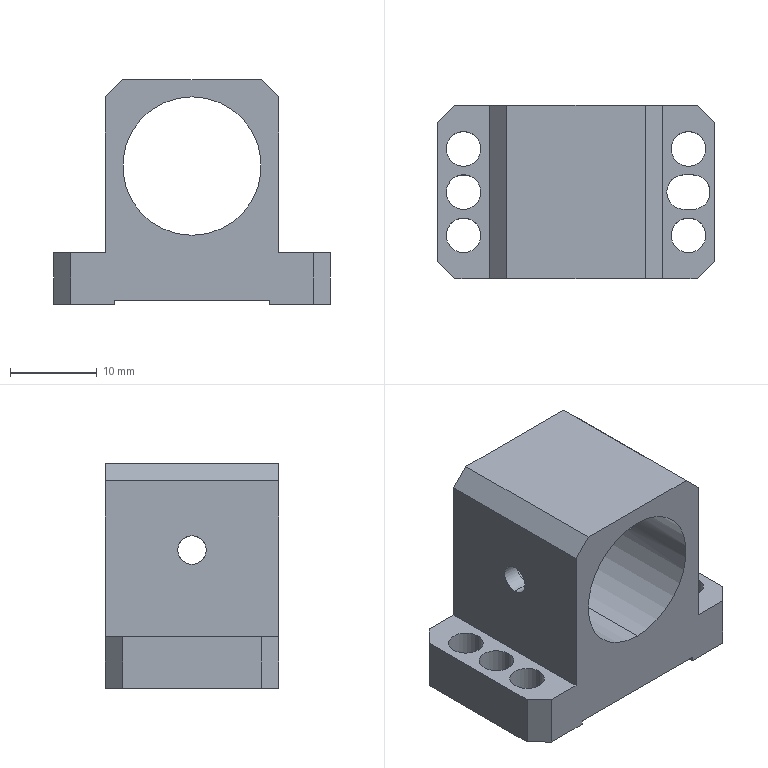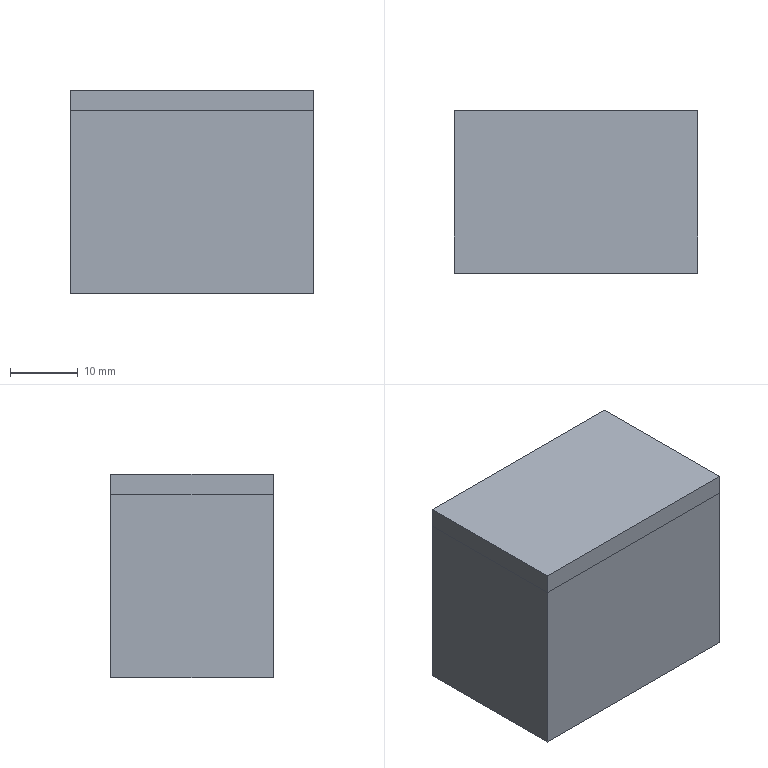CAM job | NX | 3+2 milling, drilling | part box 32 x 20 x 26 mm | stock box 36 x 24 x 30 mm
Tools:
number,name,description,diameter,corner_radius,flute_length,length,flutes
11,D10JING,Milling Tool-5 Parameters,10.0,0.0,50.0,75.0,2
10,D10,Milling Tool-5 Parameters,10.0,0.0,50.0,75.0,2
5,D4R0.5,Milling Tool-5 Parameters,4.0,0.5,50.0,75.0,2
7,D6A45,Milling Tool-5 Parameters,6.0,0.0,50.0,75.0,2
14,4.0ZT,Drilling Tool,4.0,0.0,35.0,50.0,2
3,D3,Milling Tool-5 Parameters,3.0,0.0,50.0,75.0,2
Operations:
program,operation,operation_type,tool,method,geometry_group,spindle_rpm,surface_speed,feed_per_tooth,feed_cut,feed_plunge,cut_length_mm,path_length_mm,cut_time_min,machine_time_min
1,FLOOR_WALL,VolumeBased25DMillingOperation,D10JING,METHOD,A,9500.0,298.0,0.0658,1250.0,100.0,315.997,369.997,0.2528,0.2582
1,ZLEVEL_PROFILE,ZLevelMilling,D10,METHOD,A,9500.0,298.0,0.1579,3000.0,1000.0,6899.193,6982.193,2.325,2.333
1,FLOOR_WALL_1,VolumeBased25DMillingOperation,D10,METHOD,A,9500.0,179.0,0.1316,2500.0,1000.0,4110.117,4436.557,2.005,2.037
1,ZLEVEL_PROFILE_COPY_1,ZLevelMilling,D10JING,METHOD,A,9500.0,298.0,0.0632,1200.0,1000.0,278.136,473.496,0.2331,0.2527
1,FLOOR_WALL_1_1,VolumeBased25DMillingOperation,D10JING,METHOD,A,9500.0,298.0,0.0658,1250.0,100.0,254.567,587.327,0.2037,0.2369
1,ZLEVEL_PROFILE_1,ZLevelMilling,D4R0.5,METHOD,A,9500.0,119.0,0.1579,3000.0,1000.0,1594.955,1749.084,0.5343,0.5497
1,PLANAR_MILL_COPY,PlanarMilling,D6A45,METHOD,A,9500.0,179.0,0.0658,1250.0,100.0,91.394,150.394,0.0731,0.079
1,PLANAR_MILL_COPY_COPY,PlanarMilling,D6A45,METHOD,A,9500.0,179.0,0.0658,1250.0,100.0,63.365,289.681,0.0507,0.0733
2,FLOOR_WALL_COPY,VolumeBased25DMillingOperation,D10JING,METHOD,B,9500.0,298.0,0.0658,1250.0,100.0,2527.976,3155.957,2.022,2.085
2,FLOOR_WALL_COPY_COPY,VolumeBased25DMillingOperation,D10JING,METHOD,B,9500.0,298.0,0.0658,1250.0,100.0,109.997,164.997,0.088,0.0935
2,DRILLING,Operation,D6A45,METHOD,B,5000.0,94.0,0.025,250.0,0.0,24.0,172.539,0.096,0.1109
2,DRILLING_COPY,Operation,4.0ZT,METHOD,B,2000.0,25.0,0.0625,250.0,0.0,46.807,209.667,0.1872,0.2035
2,ZLEVEL_PROFILE_COPY_COPY_1,ZLevelMilling,D3,METHOD,B,9500.0,89.0,0.0632,1200.0,1000.0,262.596,416.103,0.2265,0.2418
2,PLANAR_MILL_COPY_COPY_1_COPY,PlanarMilling,D6A45,METHOD,B,9500.0,179.0,0.0658,1250.0,100.0,173.559,718.896,0.1388,0.1934
2,PLANAR_MILL_COPY_COPY_1_COPY_COPY,PlanarMilling,D6A45,METHOD,B,9500.0,179.0,0.0658,1250.0,100.0,41.107,185.6,0.0329,0.0473
2,刀补3,ZLevelMilling,D3,METHOD,B,9500.0,89.0,0.0632,1200.0,1000.0,36.44,194.061,0.0308,0.0466
3,HOLE_MILLING,CylinderMilling,D10,METHOD,C,9500.0,298.0,0.1053,2000.0,100.0,774.684,854.184,0.3873,0.3953
3,PLANAR_MILL_COPY_COPY_1_COPY_COPY_COPY,PlanarMilling,D6A45,METHOD,C,9500.0,179.0,0.0658,1250.0,100.0,52.311,111.311,0.0418,0.0477
3,刀补,CylinderMilling,D10JING,METHOD,C,9500.0,298.0,0.0526,1000.0,100.0,106.56,186.06,0.1066,0.1145